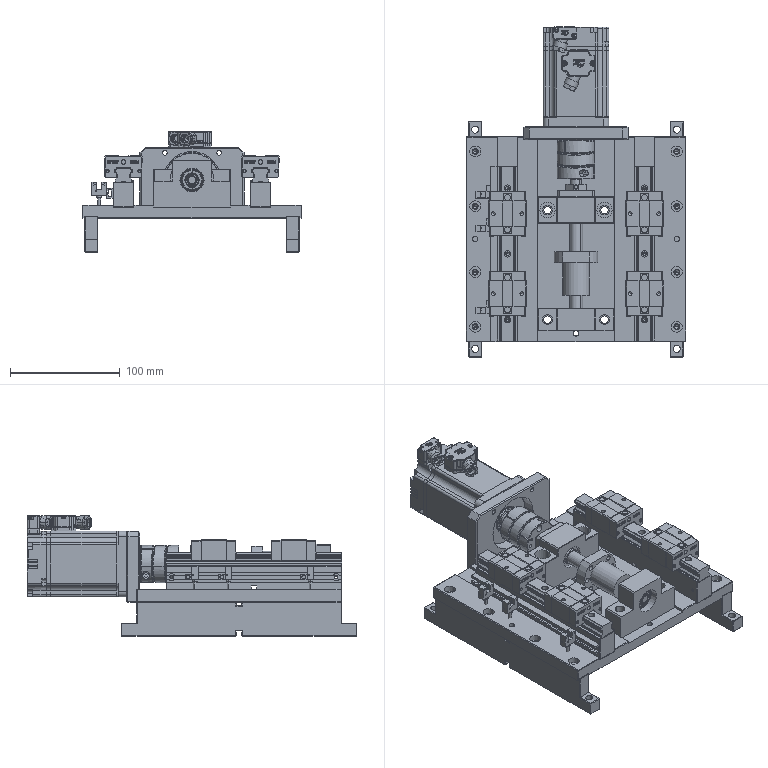Part | SolidWorks | 54 solids | 4830 faces | volume 1320917 mm3 | plane 2857 | cylinder 1151 | spline 529 | cone 195 | torus 98 | commonest cylinder face diameters 1 x119 4 x81 1.6 x64 10 x64 3 x62 2.1 x58